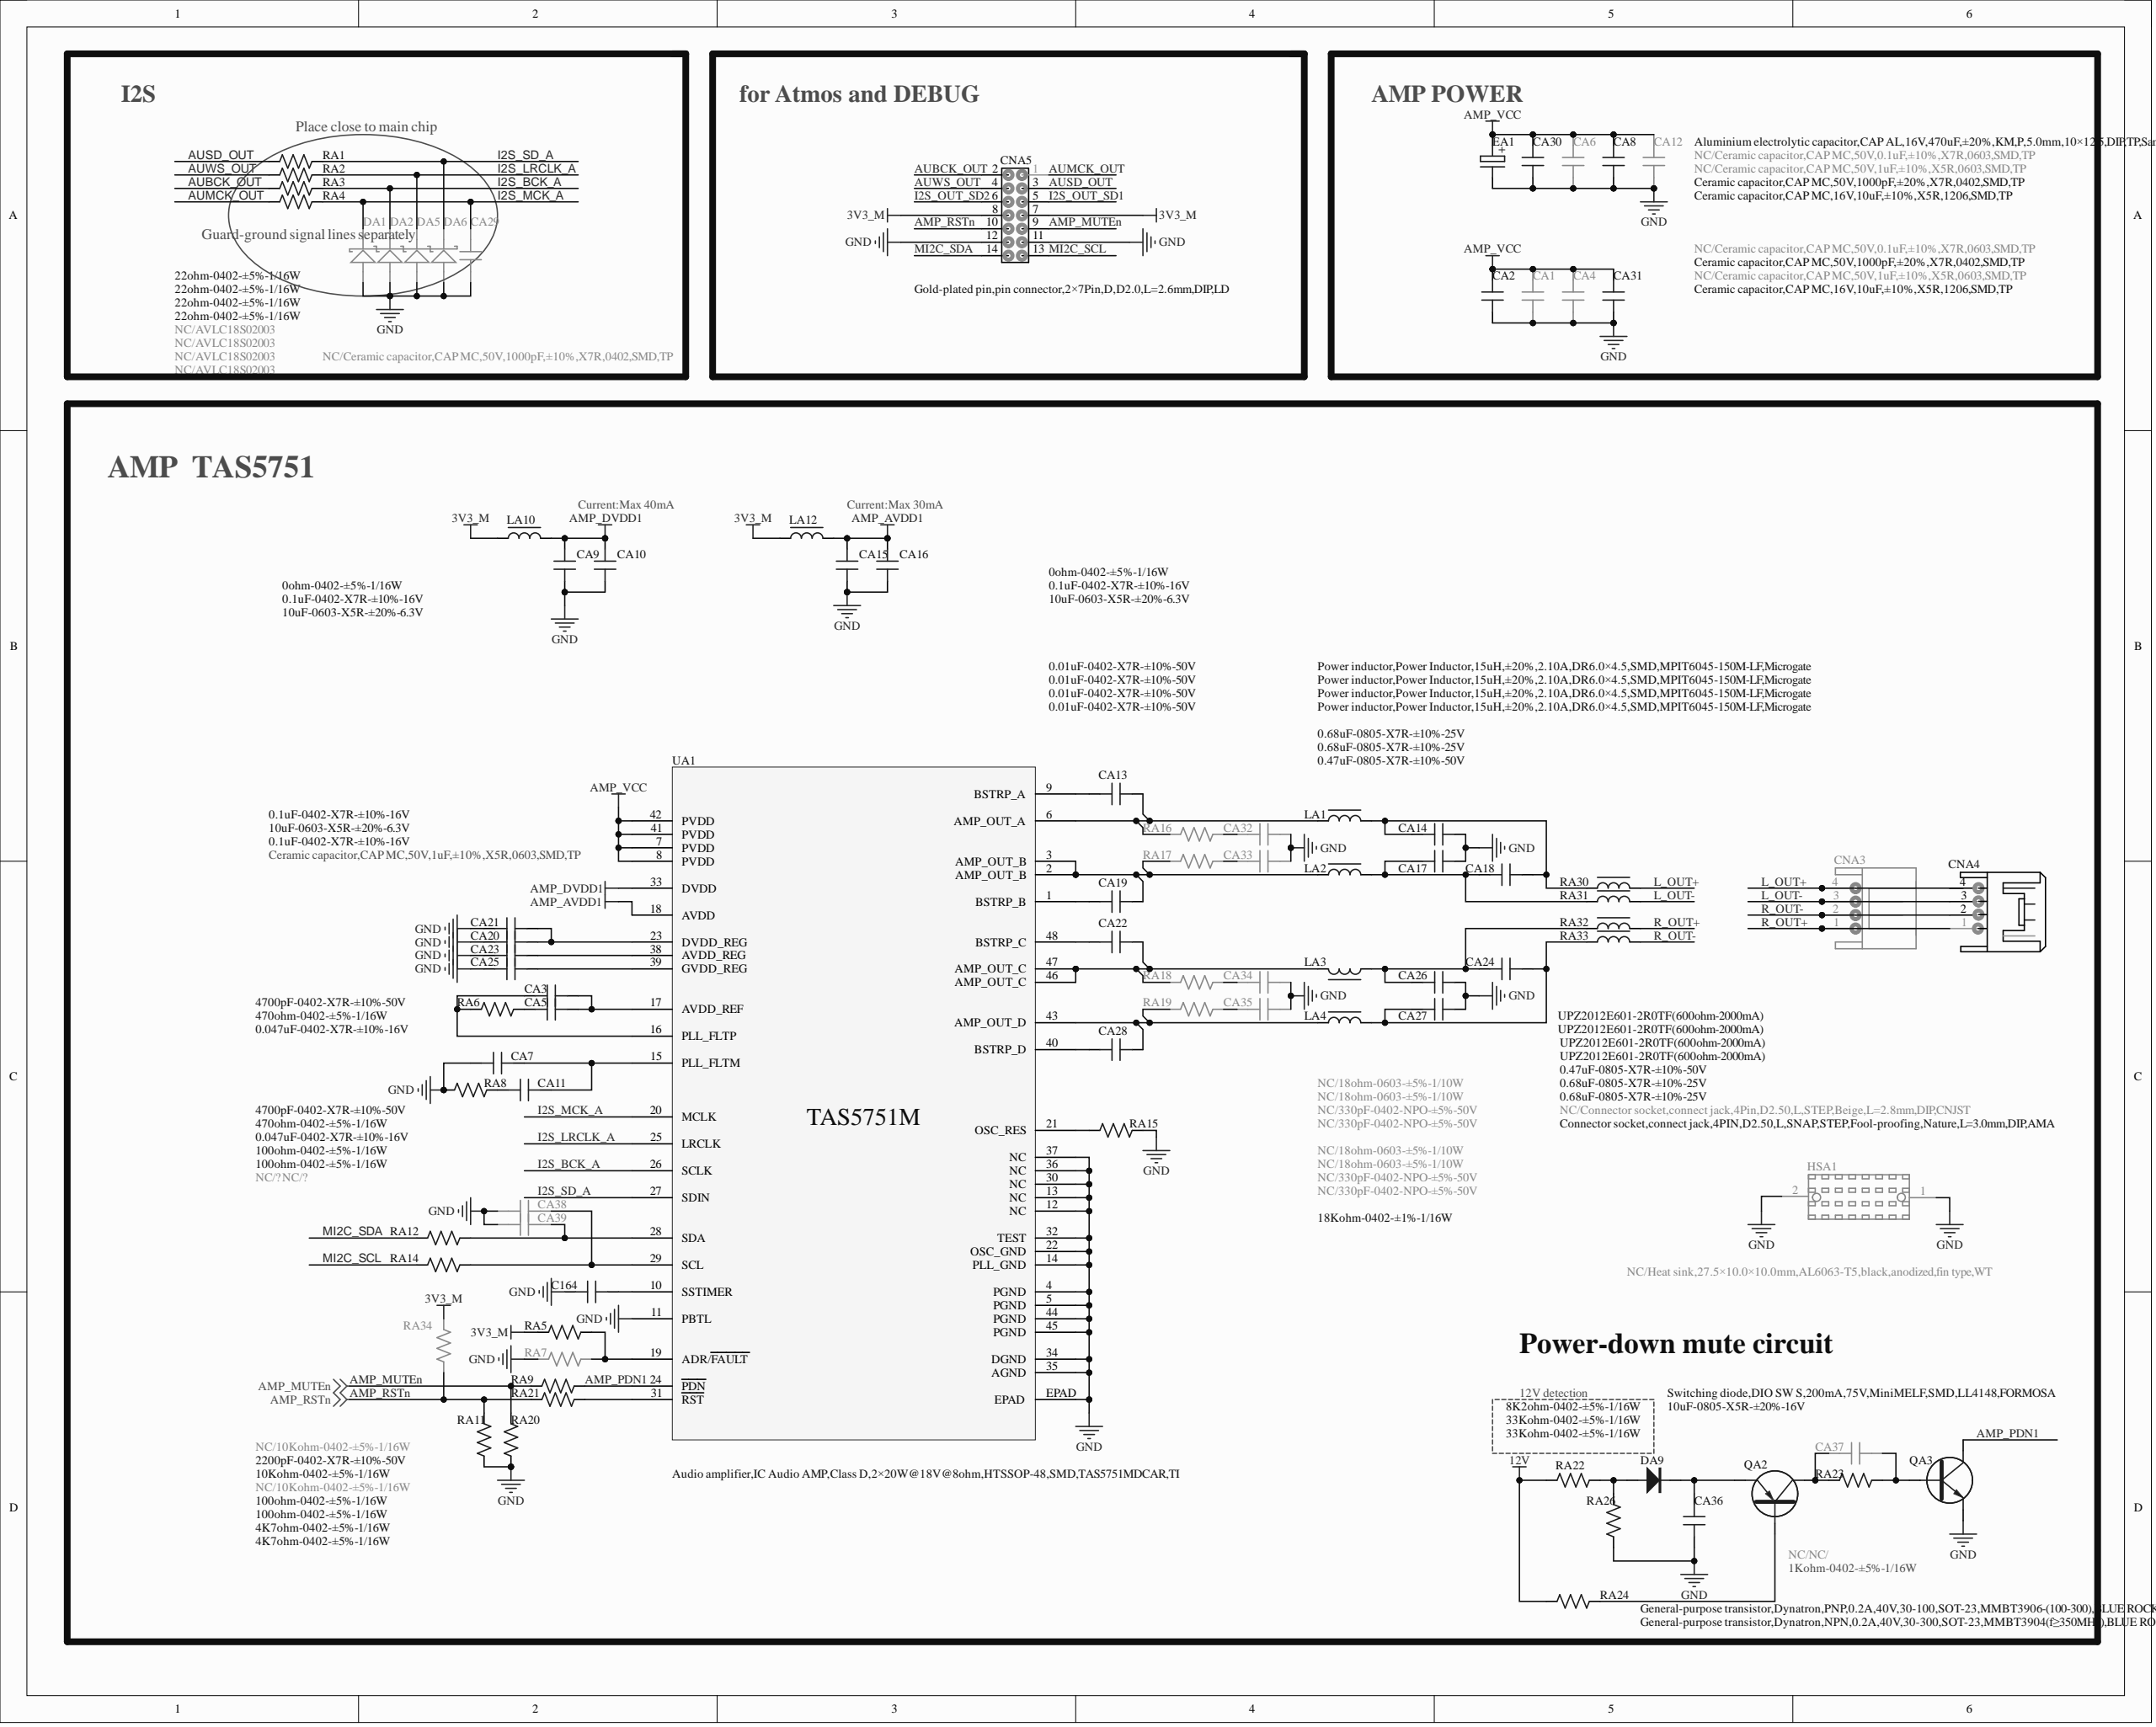Circuit board | Altium Designer | 1029 parts | 642 nets | one sheet of the schematic
Parts on this sheet (reference | value | footprint):
C164 | 2200pF-0402-X7R-±10%-50V | C0402
CA1 | NC/Ceramic capacitor,CAP MC,50V,0.1uF,±10%,X7R,0603,SMD,TP | C0603
CA2 | Ceramic capacitor,CAP MC,50V,1000pF,±20%,X7R,0402,SMD,TP | C0402
CA3 | 4700pF-0402-X7R-±10%-50V | C0402
CA4 | NC/Ceramic capacitor,CAP MC,50V,1uF,±10%,X5R,0603,SMD,TP | C0603
CA5 | 0.047uF-0402-X7R-±10%-16V | C0402
CA6 | NC/Ceramic capacitor,CAP MC,50V,0.1uF,±10%,X7R,0603,SMD,TP | C0603
CA7 | 4700pF-0402-X7R-±10%-50V | C0402
CA8 | Ceramic capacitor,CAP MC,50V,1000pF,±20%,X7R,0402,SMD,TP | C0402
CA9 | 0.1uF-0402-X7R-±10%-16V | C0402
CA10 | 10uF-0603-X5R-±20%-6.3V | C0603
CA11 | 0.047uF-0402-X7R-±10%-16V | C0402
CA12 | NC/Ceramic capacitor,CAP MC,50V,1uF,±10%,X5R,0603,SMD,TP | C0603
CA13 | 0.01uF-0402-X7R-±10%-50V | C0402
CA14 | 0.68uF-0805-X7R-±10%-25V | C0805
CA15 | 0.1uF-0402-X7R-±10%-16V | C0402
CA16 | 10uF-0603-X5R-±20%-6.3V | C0603
CA17 | 0.68uF-0805-X7R-±10%-25V | C0805
CA18 | 0.47uF-0805-X7R-±10%-50V | C0805
CA19 | 0.01uF-0402-X7R-±10%-50V | C0402
CA20 | 0.1uF-0402-X7R-±10%-16V | C0402
CA21 | 10uF-0603-X5R-±20%-6.3V | C0603
CA22 | 0.01uF-0402-X7R-±10%-50V | C0402
CA23 | 0.1uF-0402-X7R-±10%-16V | C0402
CA24 | 0.47uF-0805-X7R-±10%-50V | C0805
CA25 | Ceramic capacitor,CAP MC,50V,1uF,±10%,X5R,0603,SMD,TP | C0603
CA26 | 0.68uF-0805-X7R-±10%-25V | C0805
CA27 | 0.68uF-0805-X7R-±10%-25V | C0805
CA28 | 0.01uF-0402-X7R-±10%-50V | C0402
CA29 | NC/Ceramic capacitor,CAP MC,50V,1000pF,±10%,X7R,0402,SMD,TP | C0402
CA30 | Ceramic capacitor,CAP MC,16V,10uF,±10%,X5R,1206,SMD,TP | C1206
CA31 | Ceramic capacitor,CAP MC,16V,10uF,±10%,X5R,1206,SMD,TP | C1206
CA32 | NC/330pF-0402-NPO-±5%-50V | C0402
CA33 | NC/330pF-0402-NPO-±5%-50V | C0402
CA34 | NC/330pF-0402-NPO-±5%-50V | C0402
CA35 | NC/330pF-0402-NPO-±5%-50V | C0402
CA36 | 10uF-0805-X5R-±20%-16V | C0805
CA37 | NC/NC/ | C0402
CA38 | NC/? | C0402
CA39 | NC/? | C0402
CNA3 | NC/Connector socket,connect jack,4Pin,D2.50,L,STEP,Beige,L=2.8mm,DIP,CNJST | SIP4H/2.5D-4
CNA4 | Connector socket,connect jack,4PIN,D2.50,L,SNAP,STEP,Fool-proofing,Nature,L=3.0mm,DIP,AMA | SIP4H/2.5D-7
CNA5 | Gold-plated pin,pin connector,2×7Pin,D,D2.0,L=2.6mm,DIP,LD | SIP2*7/2.0D
DA1 | NC/AVLC18S02003 | DIODE-S0402
DA2 | NC/AVLC18S02003 | DIODE-S0402
DA5 | NC/AVLC18S02003 | DIODE-S0402
DA6 | NC/AVLC18S02003 | DIODE-S0402
DA9 | Switching diode,DIO SW S,200mA,75V,MiniMELF,SMD,LL4148,FORMOSA | DIODE-S0805
HSA1 | NC/Heat sink,27.5×10.0×10.0mm,AL6063-T5,black,anodized,fin type,WT | HS(27*10*10)-1
LA1 | Power inductor,Power Inductor,15uH,±20%,2.10A,DR6.0×4.5,SMD,MPIT6045-150M-LF,Microgate | L(6.0*4.5)-S
LA2 | Power inductor,Power Inductor,15uH,±20%,2.10A,DR6.0×4.5,SMD,MPIT6045-150M-LF,Microgate | L(6.0*4.5)-S
LA3 | Power inductor,Power Inductor,15uH,±20%,2.10A,DR6.0×4.5,SMD,MPIT6045-150M-LF,Microgate | L(6.0*4.5)-S
LA4 | Power inductor,Power Inductor,15uH,±20%,2.10A,DR6.0×4.5,SMD,MPIT6045-150M-LF,Microgate | L(6.0*4.5)-S
LA10 | 0ohm-0402-±5%-1/16W | L0402
LA12 | 0ohm-0402-±5%-1/16W | L0402
QA2 | General-purpose transistor,Dynatron,PNP,0.2A,40V,30-100,SOT-23,MMBT3906-(100-300),BLUE ROCKET | SOT-23
QA3 | General-purpose transistor,Dynatron,NPN,0.2A,40V,30-300,SOT-23,MMBT3904(f=350MHz),BLUE ROCKET | SOT-23
RA1 | 22ohm-0402-±5%-1/16W | R0402
RA2 | 22ohm-0402-±5%-1/16W | R0402
RA3 | 22ohm-0402-±5%-1/16W | R0402
RA4 | 22ohm-0402-±5%-1/16W | R0402
RA5 | 10Kohm-0402-±5%-1/16W | R0402
RA6 | 470ohm-0402-±5%-1/16W | R0402
RA7 | NC/10Kohm-0402-±5%-1/16W | R0402
RA8 | 470ohm-0402-±5%-1/16W | R0402
RA9 | 100ohm-0402-±5%-1/16W | R0402
RA11 | 4K7ohm-0402-±5%-1/16W | R0402
RA12 | 100ohm-0402-±5%-1/16W | R0402
RA14 | 100ohm-0402-±5%-1/16W | R0402
RA15 | 18Kohm-0402-±1%-1/16W | R0402
RA16 | NC/18ohm-0603-±5%-1/10W | R0603
RA17 | NC/18ohm-0603-±5%-1/10W | R0603
RA18 | NC/18ohm-0603-±5%-1/10W | R0603
RA19 | NC/18ohm-0603-±5%-1/10W | R0603
RA20 | 4K7ohm-0402-±5%-1/16W | R0402
RA21 | 100ohm-0402-±5%-1/16W | R0402
RA22 | 8K2ohm-0402-±5%-1/16W | R0402
RA23 | 1Kohm-0402-±5%-1/16W | R0402
RA24 | 33Kohm-0402-±5%-1/16W | R0402
RA26 | 33Kohm-0402-±5%-1/16W | R0402
RA30 | UPZ2012E601-2R0TF(600ohm-2000mA) | L0805
RA31 | UPZ2012E601-2R0TF(600ohm-2000mA) | L0805
RA32 | UPZ2012E601-2R0TF(600ohm-2000mA) | L0805
RA33 | UPZ2012E601-2R0TF(600ohm-2000mA) | L0805
RA34 | NC/10Kohm-0402-±5%-1/16W | R0402
UA1 | Audio amplifier,IC Audio AMP,Class D,2×20W@18V@8ohm,HTSSOP-48,SMD,TAS5751MDCAR,TI | SOP48/0.5-2
Nets of these parts (net: part-pin ...):
R_OUT-: CNA3-2 CNA4-2 RA33-2
R_OUT+: CNA3-1 CNA4-1 RA32-2
NetRA21_2: RA21-2 UA1-31
NetRA15_1: RA15-1 UA1-21
NetRA5_2: RA5-2 RA7-1 UA1-19
NetQA2_B: QA2-B RA24-1
NetDA9_A: DA9-A RA22-2 RA26-2
NetCA39_2: CA39-2 RA12-2 UA1-28
NetCA38_2: CA38-2 RA14-2 UA1-29
NetCA37_2: CA37-2 QA3-B RA23-2
NetCA37_1: CA37-1 QA2-C RA23-1
NetCA36_2: CA36-2 DA9-K QA2-E
NetCA35_1: CA35-1 RA19-2
NetCA34_1: CA34-1 RA18-2
NetCA33_1: CA33-1 RA17-2
NetCA32_1: CA32-1 RA16-2
NetCA28_2: CA28-2 LA4-1 RA19-1 UA1-43
NetCA28_1: CA28-1 UA1-40
NetCA25_1: CA25-1 UA1-39
NetCA24_2: CA24-2 CA27-1 LA4-2 RA33-1
NetCA24_1: CA24-1 CA26-1 LA3-1 RA32-1
NetCA23_1: CA23-1 UA1-38
NetCA22_2: CA22-2 LA3-2 RA18-1 UA1-46 UA1-47
NetCA22_1: CA22-1 UA1-48
NetCA20_1: CA20-1 CA21-2 UA1-23
NetCA19_2: CA19-2 LA2-1 RA17-1 UA1-2 UA1-3
NetCA19_1: CA19-1 UA1-1
NetCA17_1: CA17-1 CA18-1 LA2-2 RA31-1
NetCA14_1: CA14-1 CA18-2 LA1-2 RA30-1
NetCA13_2: CA13-2 LA1-1 RA16-1 UA1-6
NetCA13_1: CA13-1 UA1-9
NetCA11_1: CA11-1 RA8-2
NetCA7_2: CA7-2 CA11-2 UA1-15
NetCA5_1: CA5-1 RA6-2
NetCA3_2: CA3-2 CA5-2 UA1-17
NetCA3_1: CA3-1 RA6-1 UA1-16
NetC164_1: C164-1 UA1-10
MI2C_SDA: CNA5-14 RA12-1
MI2C_SCL: CNA5-13 RA14-1
L_OUT-: CNA3-3 CNA4-3 RA31-2
L_OUT+: CNA3-4 CNA4-4 RA30-2
I2S_SD_A: DA6-K RA1-2 UA1-27
I2S_OUT_SD2: CNA5-6
I2S_OUT_SD1: CNA5-5
I2S_MCK_A: CA29-2 DA1-K RA4-2 UA1-20
I2S_LRCLK_A: DA5-K RA2-2 UA1-25
I2S_BCK_A: DA2-K RA3-2 UA1-26
GND: C164-2 CA1-1 CA2-1 CA4-1 CA6-1 CA7-1 CA8-1 CA9-1 CA10-1 CA12-1 CA14-2 CA15-1 CA16-1 CA17-2 CA20-2 CA21-1 CA23-2 CA25-2 CA26-2 CA27-2 CA29-1 CA30-1 CA31-1 CA32-2 CA33-2 CA34-2 CA35-2 CA36-1 CA38-1 CA39-1 CNA5-11 CNA5-12 DA1-A DA2-A DA5-A DA6-A HSA1-1 HSA1-2 QA3-E RA7-2 RA8-1 RA11-1 RA15-2 RA20-1 RA26-1 UA1-4 UA1-5 UA1-11 UA1-12 UA1-13 UA1-14 UA1-22 UA1-30 UA1-32 UA1-34 UA1-35 UA1-36 UA1-37 UA1-44 UA1-45 UA1-EPAD
AUWS_OUT: CNA5-4 RA2-1
AUSD_OUT: CNA5-3 RA1-1
AUMCK_OUT: CNA5-1 RA4-1
AUBCK_OUT: CNA5-2 RA3-1
AMP_VCC: CA1-2 CA2-2 CA4-2 CA6-2 CA8-2 CA12-2 CA30-2 CA31-2 UA1-7 UA1-8 UA1-41 UA1-42
AMP_RSTn: CNA5-10 RA11-2 RA21-1 RA34-2
AMP_PDN1: QA3-C RA9-1 UA1-24
AMP_MUTEn: CNA5-9 RA9-2 RA20-2
AMP_DVDD1: CA9-2 CA10-2 LA10-2 UA1-33
AMP_AVDD1: CA15-2 CA16-2 LA12-2 UA1-18
12V: RA22-1 RA24-2
3V3_M: CNA5-7 CNA5-8 LA10-1 LA12-1 RA5-1 RA34-1